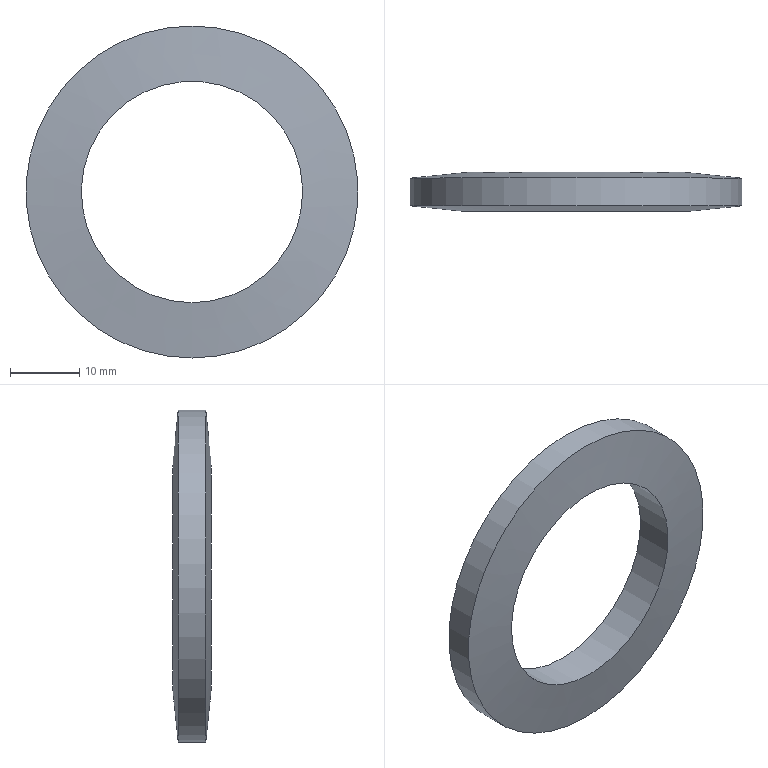Part | NX | features DATUM_CSYS 2, SKETCH 1, SWP104 1 | 1 solid | 4 faces | box 48 x 5.63 x 48 mm | volume 4786 mm3 | cone 2 | cylinder 2 | commonest cylinder face diameters 32 x1 48 x1
STEP:
#1=CARTESIAN_POINT('',(0.,-2.815,-16.));
#2=VERTEX_POINT('',#1);
#3=CARTESIAN_POINT('',(0.,-2.815,0.));
#4=DIRECTION('',(0.,-1.,0.));
#5=DIRECTION('',(0.,0.,-1.));
#6=AXIS2_PLACEMENT_3D('',#3,#4,#5);
#7=CIRCLE('',#6,16.);
#8=EDGE_CURVE('',#2,#2,#7,.T.);
#9=ORIENTED_EDGE('',*,*,#8,.F.);
#10=EDGE_LOOP('',(#9));
#11=FACE_BOUND('',#10,.T.);
#12=CARTESIAN_POINT('',(0.,-2.,-24.));
#13=VERTEX_POINT('',#12);
#14=CARTESIAN_POINT('',(0.,-2.,0.));
#15=DIRECTION('',(0.,-1.,0.));
#16=DIRECTION('',(0.,0.,-1.));
#17=AXIS2_PLACEMENT_3D('',#14,#15,#16);
#18=CIRCLE('',#17,24.);
#19=EDGE_CURVE('',#13,#13,#18,.T.);
#20=ORIENTED_EDGE('',*,*,#19,.T.);
#21=EDGE_LOOP('',(#20));
#22=FACE_BOUND('',#21,.T.);
#23=CARTESIAN_POINT('',(0.,-2.,0.));
#24=DIRECTION('',(0.,1.,0.));
#25=DIRECTION('',(0.,0.,1.));
#26=AXIS2_PLACEMENT_3D('',#23,#24,#25);
#27=CONICAL_SURFACE('',#26,24.,1.469);
#28=ADVANCED_FACE('',(#11,#22),#27,.T.);
#29=CARTESIAN_POINT('',(0.,2.815,-16.));
#30=VERTEX_POINT('',#29);
#31=CARTESIAN_POINT('',(0.,2.815,0.));
#32=DIRECTION('',(0.,-1.,0.));
#33=DIRECTION('',(0.,0.,-1.));
#34=AXIS2_PLACEMENT_3D('',#31,#32,#33);
#35=CIRCLE('',#34,16.);
#36=EDGE_CURVE('',#30,#30,#35,.T.);
#37=ORIENTED_EDGE('',*,*,#36,.F.);
#38=EDGE_LOOP('',(#37));
#39=FACE_BOUND('',#38,.T.);
#40=ORIENTED_EDGE('',*,*,#8,.T.);
#41=EDGE_LOOP('',(#40));
#42=FACE_BOUND('',#41,.T.);
#43=CARTESIAN_POINT('',(0.,0.,0.));
#44=DIRECTION('',(0.,-1.,0.));
#45=DIRECTION('',(0.,0.,-1.));
#46=AXIS2_PLACEMENT_3D('',#43,#44,#45);
#47=CYLINDRICAL_SURFACE('',#46,16.);
#48=ADVANCED_FACE('',(#39,#42),#47,.F.);
#49=CARTESIAN_POINT('',(0.,2.,-24.));
#50=VERTEX_POINT('',#49);
#51=CARTESIAN_POINT('',(0.,2.,0.));
#52=DIRECTION('',(0.,-1.,0.));
#53=DIRECTION('',(0.,0.,-1.));
#54=AXIS2_PLACEMENT_3D('',#51,#52,#53);
#55=CIRCLE('',#54,24.);
#56=EDGE_CURVE('',#50,#50,#55,.T.);
#57=ORIENTED_EDGE('',*,*,#56,.F.);
#58=EDGE_LOOP('',(#57));
#59=FACE_BOUND('',#58,.T.);
#60=ORIENTED_EDGE('',*,*,#36,.T.);
#61=EDGE_LOOP('',(#60));
#62=FACE_BOUND('',#61,.T.);
#63=CARTESIAN_POINT('',(0.,2.815,0.));
#64=DIRECTION('',(0.,-1.,0.));
#65=DIRECTION('',(0.,0.,-1.));
#66=AXIS2_PLACEMENT_3D('',#63,#64,#65);
#67=CONICAL_SURFACE('',#66,16.,1.469);
#68=ADVANCED_FACE('',(#59,#62),#67,.T.);
#69=ORIENTED_EDGE('',*,*,#19,.F.);
#70=EDGE_LOOP('',(#69));
#71=FACE_BOUND('',#70,.T.);
#72=ORIENTED_EDGE('',*,*,#56,.T.);
#73=EDGE_LOOP('',(#72));
#74=FACE_BOUND('',#73,.T.);
#75=CARTESIAN_POINT('',(0.,0.,0.));
#76=DIRECTION('',(0.,-1.,0.));
#77=DIRECTION('',(0.,0.,-1.));
#78=AXIS2_PLACEMENT_3D('',#75,#76,#77);
#79=CYLINDRICAL_SURFACE('',#78,24.);
#80=ADVANCED_FACE('',(#71,#74),#79,.T.);
#81=CLOSED_SHELL('',(#28,#48,#68,#80));
#82=MANIFOLD_SOLID_BREP('',#81);
#83=(LENGTH_UNIT()NAMED_UNIT(*)SI_UNIT(.MILLI.,.METRE.));
#84=UNCERTAINTY_MEASURE_WITH_UNIT(LENGTH_MEASURE(0.00001),#83,'','');
#85=(NAMED_UNIT(*)PLANE_ANGLE_UNIT()SI_UNIT($,.RADIAN.));
#86=(NAMED_UNIT(*)SI_UNIT($,.STERADIAN.)SOLID_ANGLE_UNIT());
#87=(GEOMETRIC_REPRESENTATION_CONTEXT(3)GLOBAL_UNCERTAINTY_ASSIGNED_CONTEXT((#84))GLOBAL_UNIT_ASSIGNED_CONTEXT((#83,#85,#86))REPRESENTATION_CONTEXT('',''));
#88=ADVANCED_BREP_SHAPE_REPRESENTATION('',(#82),#87);